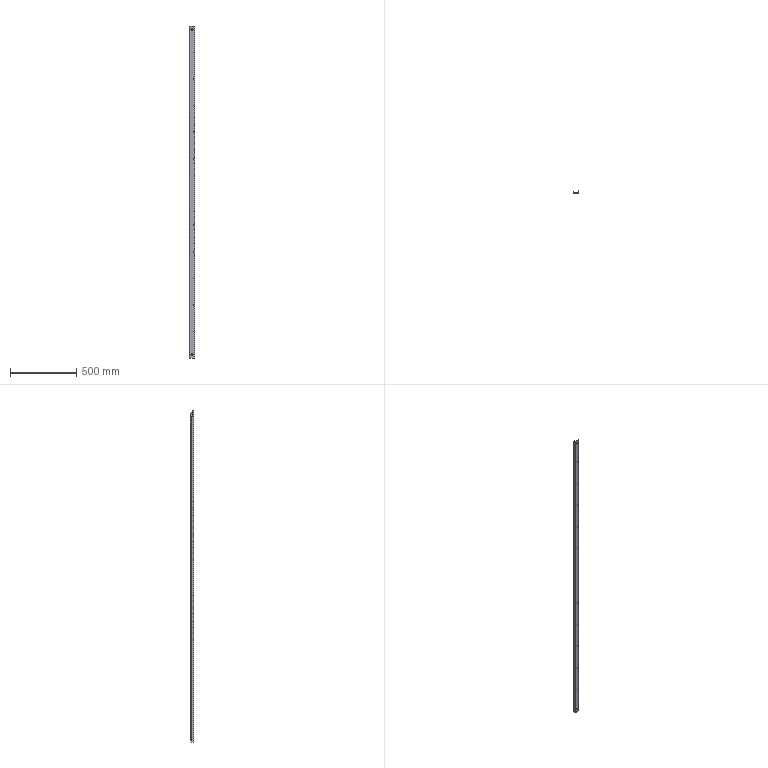Part | SolidWorks | features ICE 3, Chamfer 2, Cut 2, FlatPattern 1, SMBaseFlange 1, SheetMetal 1 | 1 solid | 97 faces | box 40 x 25 x 2501 mm | volume 530573 mm3 | cylinder 54 | plane 43 | commonest cylinder face diameters 8 x28 4.2 x20 11 x4 2 x2